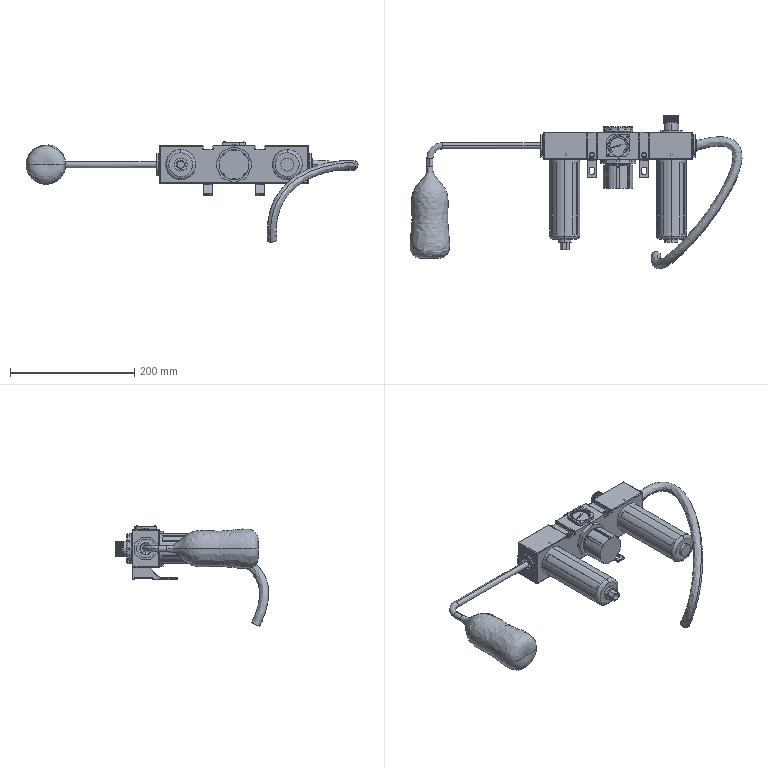Part | STEP file | GC300-400 FRL air unit [GC400-15]_GC400-15 | 2 solids | 956 faces | box 534.272 x 247.073 x 161.659 mm | volume 1621507 mm3 | plane 559 | cylinder 247 | spline 115 | cone 33 | torus 2 | commonest cylinder face diameters 2 x89 0.6 x44 42.169 x15 0.851 x12 45.769 x9 4 x8